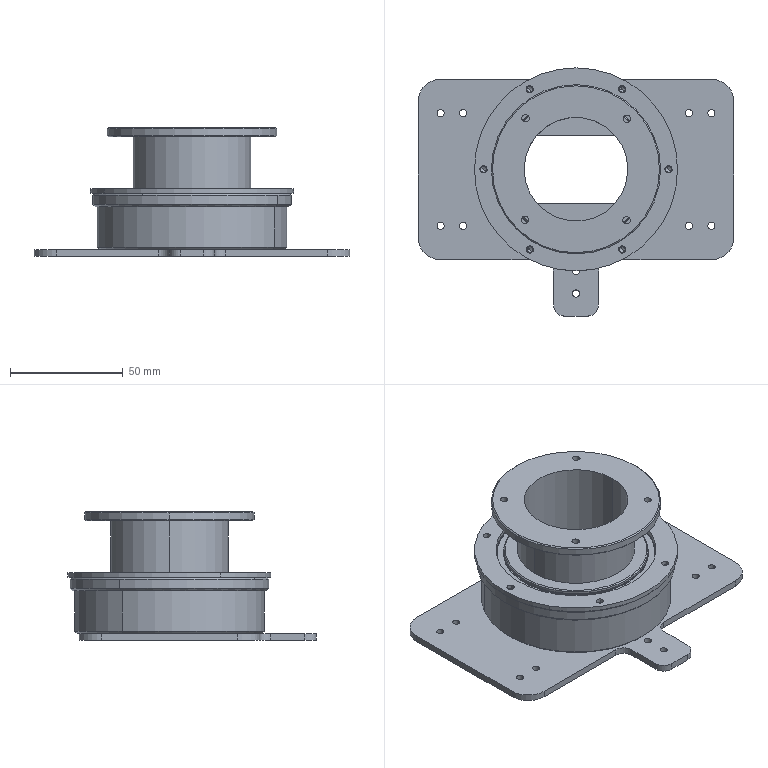Part | SolidWorks | 6 solids | 259 faces | box 140 x 110 x 57 mm | volume 121657 mm3 | cylinder 162 | cone 60 | plane 37 | commonest cylinder face diameters 3.2 x60 2.5 x36 3.3 x8 10 x8 64 x6 20 x4